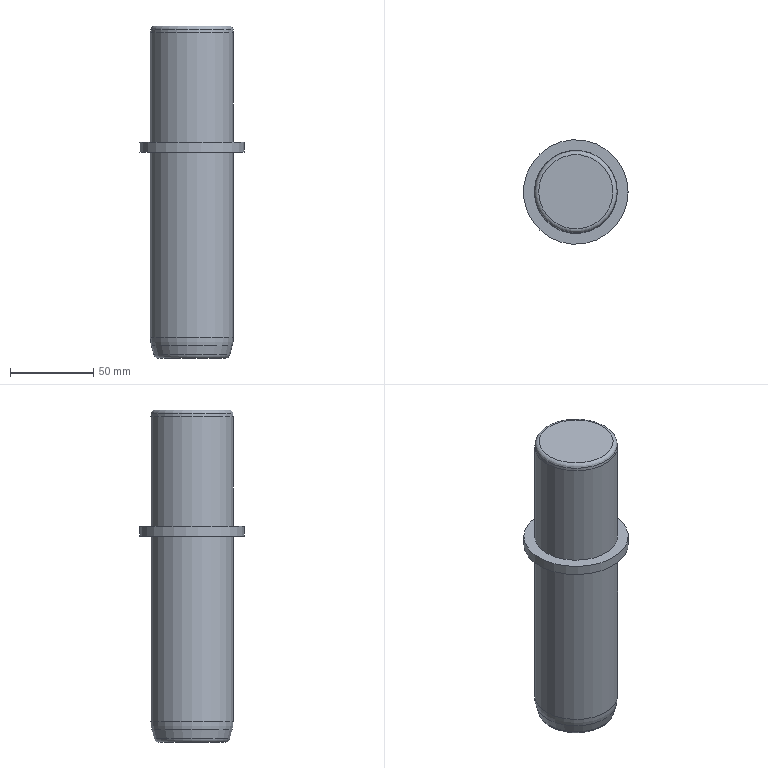Part | NX | features MAIN_BODY 2 | 1 solid | 12 faces | box 63 x 63 x 200 mm | volume 397223 mm3 | plane 4 | cylinder 3 | torus 3 | cone 2 | commonest cylinder face diameters 50 x2 63 x1
STEP:
#1=CARTESIAN_POINT('',(1045.,230.,157.504));
#2=VERTEX_POINT('',#1);
#3=CARTESIAN_POINT('',(1020.,230.,157.504));
#4=DIRECTION('',(0.,0.,1.));
#5=DIRECTION('',(1.,0.,0.));
#6=AXIS2_PLACEMENT_3D('',#3,#4,#5);
#7=CIRCLE('',#6,25.);
#8=EDGE_CURVE('',#2,#2,#7,.F.);
#9=ORIENTED_EDGE('',*,*,#8,.F.);
#10=EDGE_LOOP('',(#9));
#11=FACE_BOUND('',#10,.T.);
#12=CARTESIAN_POINT('',(1045.,230.,269.));
#13=VERTEX_POINT('',#12);
#14=CARTESIAN_POINT('',(1020.,230.,269.));
#15=DIRECTION('',(0.,0.,1.));
#16=DIRECTION('',(1.,0.,0.));
#17=AXIS2_PLACEMENT_3D('',#14,#15,#16);
#18=CIRCLE('',#17,25.);
#19=EDGE_CURVE('',#13,#13,#18,.T.);
#20=ORIENTED_EDGE('',*,*,#19,.F.);
#21=EDGE_LOOP('',(#20));
#22=FACE_BOUND('',#21,.T.);
#23=CARTESIAN_POINT('',(1020.,230.,145.));
#24=DIRECTION('',(0.,0.,1.));
#25=DIRECTION('',(-1.,0.,0.));
#26=AXIS2_PLACEMENT_3D('',#23,#24,#25);
#27=CYLINDRICAL_SURFACE('',#26,25.);
#28=ADVANCED_FACE('',(#11,#22),#27,.T.);
#29=CARTESIAN_POINT('',(1040.437,230.,145.));
#30=VERTEX_POINT('',#29);
#31=CARTESIAN_POINT('',(1020.,230.,145.));
#32=DIRECTION('',(0.,0.,1.));
#33=DIRECTION('',(1.,0.,0.));
#34=AXIS2_PLACEMENT_3D('',#31,#32,#33);
#35=CIRCLE('',#34,20.437);
#36=EDGE_CURVE('',#30,#30,#35,.T.);
#37=ORIENTED_EDGE('',*,*,#36,.F.);
#38=EDGE_LOOP('',(#37));
#39=FACE_BOUND('',#38,.T.);
#40=CARTESIAN_POINT('',(1020.,230.,145.));
#41=DIRECTION('',(0.,0.,-1.));
#42=DIRECTION('',(1.,0.,0.));
#43=AXIS2_PLACEMENT_3D('',#40,#41,#42);
#44=PLANE('',#43);
#45=ADVANCED_FACE('',(#39),#44,.T.);
#46=CARTESIAN_POINT('',(1051.5,230.,269.));
#47=VERTEX_POINT('',#46);
#48=CARTESIAN_POINT('',(1020.,230.,269.));
#49=DIRECTION('',(0.,0.,1.));
#50=DIRECTION('',(1.,0.,0.));
#51=AXIS2_PLACEMENT_3D('',#48,#49,#50);
#52=CIRCLE('',#51,31.5);
#53=EDGE_CURVE('',#47,#47,#52,.T.);
#54=ORIENTED_EDGE('',*,*,#53,.F.);
#55=EDGE_LOOP('',(#54));
#56=FACE_BOUND('',#55,.T.);
#57=ORIENTED_EDGE('',*,*,#19,.T.);
#58=EDGE_LOOP('',(#57));
#59=FACE_BOUND('',#58,.T.);
#60=CARTESIAN_POINT('',(1020.,230.,269.));
#61=DIRECTION('',(0.,0.,-1.));
#62=DIRECTION('',(1.,0.,0.));
#63=AXIS2_PLACEMENT_3D('',#60,#61,#62);
#64=PLANE('',#63);
#65=ADVANCED_FACE('',(#56,#59),#64,.T.);
#66=CARTESIAN_POINT('',(1051.5,230.,275.));
#67=VERTEX_POINT('',#66);
#68=CARTESIAN_POINT('',(1020.,230.,275.));
#69=DIRECTION('',(0.,0.,1.));
#70=DIRECTION('',(1.,0.,0.));
#71=AXIS2_PLACEMENT_3D('',#68,#69,#70);
#72=CIRCLE('',#71,31.5);
#73=EDGE_CURVE('',#67,#67,#72,.T.);
#74=ORIENTED_EDGE('',*,*,#73,.T.);
#75=EDGE_LOOP('',(#74));
#76=FACE_BOUND('',#75,.T.);
#77=CARTESIAN_POINT('',(1045.,230.,275.));
#78=VERTEX_POINT('',#77);
#79=CARTESIAN_POINT('',(1020.,230.,275.));
#80=DIRECTION('',(0.,0.,1.));
#81=DIRECTION('',(1.,0.,0.));
#82=AXIS2_PLACEMENT_3D('',#79,#80,#81);
#83=CIRCLE('',#82,25.);
#84=EDGE_CURVE('',#78,#78,#83,.T.);
#85=ORIENTED_EDGE('',*,*,#84,.F.);
#86=EDGE_LOOP('',(#85));
#87=FACE_BOUND('',#86,.T.);
#88=CARTESIAN_POINT('',(1020.,230.,275.));
#89=DIRECTION('',(0.,0.,-1.));
#90=DIRECTION('',(1.,0.,0.));
#91=AXIS2_PLACEMENT_3D('',#88,#89,#90);
#92=PLANE('',#91);
#93=ADVANCED_FACE('',(#76,#87),#92,.F.);
#94=ORIENTED_EDGE('',*,*,#53,.T.);
#95=EDGE_LOOP('',(#94));
#96=FACE_BOUND('',#95,.T.);
#97=ORIENTED_EDGE('',*,*,#73,.F.);
#98=EDGE_LOOP('',(#97));
#99=FACE_BOUND('',#98,.T.);
#100=CARTESIAN_POINT('',(1020.,230.,269.));
#101=DIRECTION('',(0.,0.,1.));
#102=DIRECTION('',(-1.,0.,0.));
#103=AXIS2_PLACEMENT_3D('',#100,#101,#102);
#104=CYLINDRICAL_SURFACE('',#103,31.5);
#105=ADVANCED_FACE('',(#96,#99),#104,.T.);
#106=CARTESIAN_POINT('',(1042.359,230.,345.));
#107=VERTEX_POINT('',#106);
#108=CARTESIAN_POINT('',(1020.,230.,345.));
#109=DIRECTION('',(0.,0.,1.));
#110=DIRECTION('',(1.,0.,0.));
#111=AXIS2_PLACEMENT_3D('',#108,#109,#110);
#112=CIRCLE('',#111,22.359);
#113=EDGE_CURVE('',#107,#107,#112,.F.);
#114=ORIENTED_EDGE('',*,*,#113,.F.);
#115=EDGE_LOOP('',(#114));
#116=FACE_BOUND('',#115,.T.);
#117=CARTESIAN_POINT('',(1020.,230.,345.));
#118=DIRECTION('',(0.,0.,-1.));
#119=DIRECTION('',(1.,0.,0.));
#120=AXIS2_PLACEMENT_3D('',#117,#118,#119);
#121=PLANE('',#120);
#122=ADVANCED_FACE('',(#116),#121,.F.);
#123=CARTESIAN_POINT('',(1045.,230.,341.));
#124=VERTEX_POINT('',#123);
#125=CARTESIAN_POINT('',(1020.,230.,341.));
#126=DIRECTION('',(0.,0.,1.));
#127=DIRECTION('',(1.,0.,0.));
#128=AXIS2_PLACEMENT_3D('',#125,#126,#127);
#129=CIRCLE('',#128,25.);
#130=EDGE_CURVE('',#124,#124,#129,.T.);
#131=ORIENTED_EDGE('',*,*,#130,.F.);
#132=EDGE_LOOP('',(#131));
#133=FACE_BOUND('',#132,.T.);
#134=ORIENTED_EDGE('',*,*,#84,.T.);
#135=EDGE_LOOP('',(#134));
#136=FACE_BOUND('',#135,.T.);
#137=CARTESIAN_POINT('',(1020.,230.,145.));
#138=DIRECTION('',(0.,0.,1.));
#139=DIRECTION('',(-1.,0.,0.));
#140=AXIS2_PLACEMENT_3D('',#137,#138,#139);
#141=CYLINDRICAL_SURFACE('',#140,25.);
#142=ADVANCED_FACE('',(#133,#136),#141,.T.);
#143=CARTESIAN_POINT('',(1042.852,230.,146.853));
#144=VERTEX_POINT('',#143);
#145=CARTESIAN_POINT('',(1020.,230.,146.853));
#146=DIRECTION('',(0.,0.,1.));
#147=DIRECTION('',(1.,0.,0.));
#148=AXIS2_PLACEMENT_3D('',#145,#146,#147);
#149=CIRCLE('',#148,22.852);
#150=EDGE_CURVE('',#144,#144,#149,.F.);
#151=ORIENTED_EDGE('',*,*,#150,.F.);
#152=EDGE_LOOP('',(#151));
#153=FACE_BOUND('',#152,.T.);
#154=CARTESIAN_POINT('',(995.681,230.,152.328));
#155=VERTEX_POINT('',#154);
#156=CARTESIAN_POINT('',(1020.,230.,152.328));
#157=DIRECTION('',(0.,0.,-1.));
#158=DIRECTION('',(-1.,0.,0.));
#159=AXIS2_PLACEMENT_3D('',#156,#157,#158);
#160=CIRCLE('',#159,24.319);
#161=EDGE_CURVE('',#155,#155,#160,.F.);
#162=ORIENTED_EDGE('',*,*,#161,.F.);
#163=EDGE_LOOP('',(#162));
#164=FACE_BOUND('',#163,.T.);
#165=CARTESIAN_POINT('',(1020.,230.,145.));
#166=DIRECTION('',(0.,0.,1.));
#167=DIRECTION('',(-1.,0.,0.));
#168=AXIS2_PLACEMENT_3D('',#165,#166,#167);
#169=CONICAL_SURFACE('',#168,22.355,0.2618);
#170=ADVANCED_FACE('',(#153,#164),#169,.T.);
#171=CARTESIAN_POINT('',(1044.85,230.,342.718));
#172=VERTEX_POINT('',#171);
#173=CARTESIAN_POINT('',(1020.,230.,342.718));
#174=DIRECTION('',(0.,0.,1.));
#175=DIRECTION('',(1.,0.,0.));
#176=AXIS2_PLACEMENT_3D('',#173,#174,#175);
#177=CIRCLE('',#176,24.85);
#178=EDGE_CURVE('',#172,#172,#177,.T.);
#179=ORIENTED_EDGE('',*,*,#178,.F.);
#180=EDGE_LOOP('',(#179));
#181=FACE_BOUND('',#180,.T.);
#182=ORIENTED_EDGE('',*,*,#130,.T.);
#183=EDGE_LOOP('',(#182));
#184=FACE_BOUND('',#183,.T.);
#185=CARTESIAN_POINT('',(1020.,230.,341.));
#186=DIRECTION('',(0.,0.,-1.));
#187=DIRECTION('',(1.,0.,0.));
#188=AXIS2_PLACEMENT_3D('',#185,#186,#187);
#189=CONICAL_SURFACE('',#188,25.,0.08727);
#190=ADVANCED_FACE('',(#181,#184),#189,.T.);
#191=ORIENTED_EDGE('',*,*,#161,.T.);
#192=EDGE_LOOP('',(#191));
#193=FACE_BOUND('',#192,.T.);
#194=ORIENTED_EDGE('',*,*,#8,.T.);
#195=EDGE_LOOP('',(#194));
#196=FACE_BOUND('',#195,.T.);
#197=CARTESIAN_POINT('',(1020.,230.,157.504));
#198=DIRECTION('',(0.,0.,-1.));
#199=DIRECTION('',(1.,0.,0.));
#200=AXIS2_PLACEMENT_3D('',#197,#198,#199);
#201=DEGENERATE_TOROIDAL_SURFACE('',#200,5.,20.,.T.);
#202=ADVANCED_FACE('',(#193,#196),#201,.T.);
#203=ORIENTED_EDGE('',*,*,#178,.T.);
#204=EDGE_LOOP('',(#203));
#205=FACE_BOUND('',#204,.T.);
#206=ORIENTED_EDGE('',*,*,#113,.T.);
#207=EDGE_LOOP('',(#206));
#208=FACE_BOUND('',#207,.T.);
#209=CARTESIAN_POINT('',(1020.,230.,342.5));
#210=DIRECTION('',(0.,0.,-1.));
#211=DIRECTION('',(1.,0.,0.));
#212=AXIS2_PLACEMENT_3D('',#209,#210,#211);
#213=TOROIDAL_SURFACE('',#212,22.359,2.5);
#214=ADVANCED_FACE('',(#205,#208),#213,.T.);
#215=ORIENTED_EDGE('',*,*,#150,.T.);
#216=EDGE_LOOP('',(#215));
#217=FACE_BOUND('',#216,.T.);
#218=ORIENTED_EDGE('',*,*,#36,.T.);
#219=EDGE_LOOP('',(#218));
#220=FACE_BOUND('',#219,.T.);
#221=CARTESIAN_POINT('',(1020.,230.,147.5));
#222=DIRECTION('',(0.,0.,-1.));
#223=DIRECTION('',(1.,0.,0.));
#224=AXIS2_PLACEMENT_3D('',#221,#222,#223);
#225=TOROIDAL_SURFACE('',#224,20.437,2.5);
#226=ADVANCED_FACE('',(#217,#220),#225,.T.);
#227=CLOSED_SHELL('',(#28,#45,#65,#93,#105,#122,#142,#170,#190,#202,#214,#226));
#228=MANIFOLD_SOLID_BREP('',#227);
#229=(LENGTH_UNIT()NAMED_UNIT(*)SI_UNIT(.MILLI.,.METRE.));
#230=UNCERTAINTY_MEASURE_WITH_UNIT(LENGTH_MEASURE(0.00001),#229,'','');
#231=(NAMED_UNIT(*)PLANE_ANGLE_UNIT()SI_UNIT($,.RADIAN.));
#232=(NAMED_UNIT(*)SI_UNIT($,.STERADIAN.)SOLID_ANGLE_UNIT());
#233=(GEOMETRIC_REPRESENTATION_CONTEXT(3)GLOBAL_UNCERTAINTY_ASSIGNED_CONTEXT((#230))GLOBAL_UNIT_ASSIGNED_CONTEXT((#229,#231,#232))REPRESENTATION_CONTEXT('',''));
#234=ADVANCED_BREP_SHAPE_REPRESENTATION('',(#228),#233);